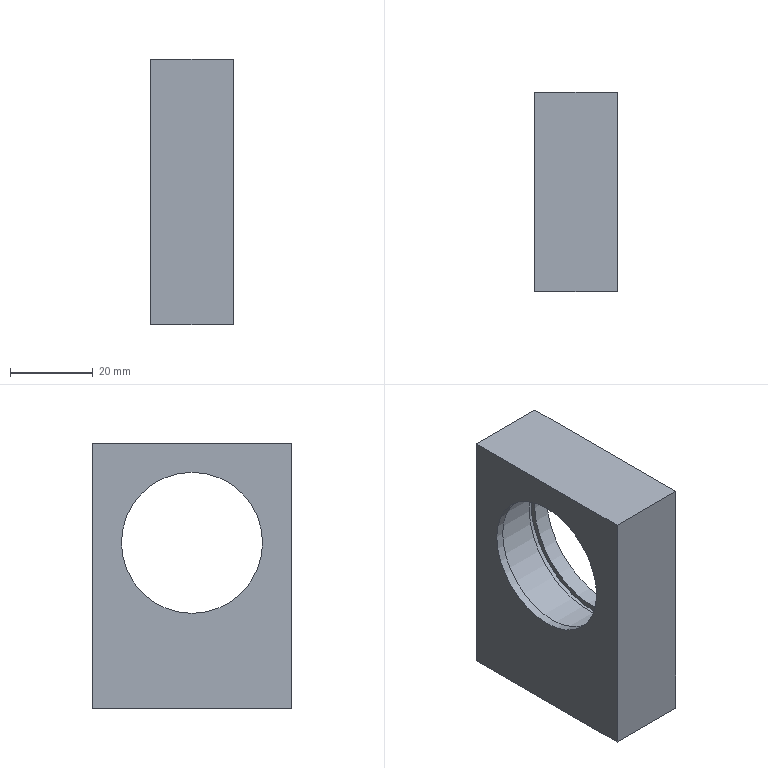Part | NX | features Housing_5003_010_BGBKB6203ZZ-40 2 | 1 solid | 17 faces | box 20 x 48 x 64 mm | volume 36127 mm3 | plane 9 | cylinder 6 | cone 2 | commonest cylinder face diameters 5 x2 40 x2 34 x1 42.5 x1
STEP:
#1=CARTESIAN_POINT('',(171.525,100.,-123.));
#2=VERTEX_POINT('',#1);
#3=CARTESIAN_POINT('',(171.525,100.,-187.));
#4=VERTEX_POINT('',#3);
#5=CARTESIAN_POINT('',(171.525,100.,-187.));
#6=DIRECTION('',(0.,0.,-1.));
#7=VECTOR('',#6,1000.);
#8=LINE('',#5,#7);
#9=EDGE_CURVE('',#2,#4,#8,.T.);
#10=ORIENTED_EDGE('',*,*,#9,.T.);
#11=CARTESIAN_POINT('',(191.525,100.,-187.));
#12=VERTEX_POINT('',#11);
#13=CARTESIAN_POINT('',(191.525,100.,-187.));
#14=DIRECTION('',(-1.,0.,0.));
#15=VECTOR('',#14,1000.);
#16=LINE('',#13,#15);
#17=EDGE_CURVE('',#12,#4,#16,.T.);
#18=ORIENTED_EDGE('',*,*,#17,.F.);
#19=CARTESIAN_POINT('',(191.525,100.,-123.));
#20=VERTEX_POINT('',#19);
#21=CARTESIAN_POINT('',(191.525,100.,-187.));
#22=DIRECTION('',(0.,0.,-1.));
#23=VECTOR('',#22,1000.);
#24=LINE('',#21,#23);
#25=EDGE_CURVE('',#20,#12,#24,.T.);
#26=ORIENTED_EDGE('',*,*,#25,.F.);
#27=CARTESIAN_POINT('',(191.525,100.,-123.));
#28=DIRECTION('',(-1.,0.,0.));
#29=VECTOR('',#28,1000.);
#30=LINE('',#27,#29);
#31=EDGE_CURVE('',#20,#2,#30,.T.);
#32=ORIENTED_EDGE('',*,*,#31,.T.);
#33=EDGE_LOOP('',(#10,#18,#26,#32));
#34=FACE_BOUND('',#33,.T.);
#35=CARTESIAN_POINT('',(191.525,100.,-187.));
#36=DIRECTION('',(0.,1.,0.));
#37=DIRECTION('',(-1.,0.,0.));
#38=AXIS2_PLACEMENT_3D('',#35,#36,#37);
#39=PLANE('',#38);
#40=ADVANCED_FACE('',(#34),#39,.F.);
#41=CARTESIAN_POINT('',(179.025,142.,-187.));
#42=VERTEX_POINT('',#41);
#43=CARTESIAN_POINT('',(181.525,142.,-187.));
#44=DIRECTION('',(0.,0.,-1.));
#45=DIRECTION('',(-1.,0.,0.));
#46=AXIS2_PLACEMENT_3D('',#43,#44,#45);
#47=CIRCLE('',#46,2.5);
#48=EDGE_CURVE('',#42,#42,#47,.T.);
#49=ORIENTED_EDGE('',*,*,#48,.F.);
#50=EDGE_LOOP('',(#49));
#51=FACE_BOUND('',#50,.T.);
#52=CARTESIAN_POINT('',(179.025,106.,-187.));
#53=VERTEX_POINT('',#52);
#54=CARTESIAN_POINT('',(181.525,106.,-187.));
#55=DIRECTION('',(0.,0.,-1.));
#56=DIRECTION('',(-1.,0.,0.));
#57=AXIS2_PLACEMENT_3D('',#54,#55,#56);
#58=CIRCLE('',#57,2.5);
#59=EDGE_CURVE('',#53,#53,#58,.T.);
#60=ORIENTED_EDGE('',*,*,#59,.F.);
#61=EDGE_LOOP('',(#60));
#62=FACE_BOUND('',#61,.T.);
#63=CARTESIAN_POINT('',(171.525,148.,-187.));
#64=VERTEX_POINT('',#63);
#65=CARTESIAN_POINT('',(171.525,100.,-187.));
#66=DIRECTION('',(0.,1.,0.));
#67=VECTOR('',#66,1000.);
#68=LINE('',#65,#67);
#69=EDGE_CURVE('',#4,#64,#68,.T.);
#70=ORIENTED_EDGE('',*,*,#69,.T.);
#71=CARTESIAN_POINT('',(191.525,148.,-187.));
#72=VERTEX_POINT('',#71);
#73=CARTESIAN_POINT('',(191.525,148.,-187.));
#74=DIRECTION('',(-1.,0.,0.));
#75=VECTOR('',#74,1000.);
#76=LINE('',#73,#75);
#77=EDGE_CURVE('',#72,#64,#76,.T.);
#78=ORIENTED_EDGE('',*,*,#77,.F.);
#79=CARTESIAN_POINT('',(191.525,100.,-187.));
#80=DIRECTION('',(0.,1.,0.));
#81=VECTOR('',#80,1000.);
#82=LINE('',#79,#81);
#83=EDGE_CURVE('',#12,#72,#82,.T.);
#84=ORIENTED_EDGE('',*,*,#83,.F.);
#85=ORIENTED_EDGE('',*,*,#17,.T.);
#86=EDGE_LOOP('',(#70,#78,#84,#85));
#87=FACE_BOUND('',#86,.T.);
#88=CARTESIAN_POINT('',(191.525,100.,-187.));
#89=DIRECTION('',(0.,0.,1.));
#90=DIRECTION('',(1.,0.,0.));
#91=AXIS2_PLACEMENT_3D('',#88,#89,#90);
#92=PLANE('',#91);
#93=ADVANCED_FACE('',(#51,#62,#87),#92,.F.);
#94=CARTESIAN_POINT('',(171.525,148.,-123.));
#95=VERTEX_POINT('',#94);
#96=CARTESIAN_POINT('',(171.525,148.,-187.));
#97=DIRECTION('',(0.,0.,1.));
#98=VECTOR('',#97,1000.);
#99=LINE('',#96,#98);
#100=EDGE_CURVE('',#64,#95,#99,.T.);
#101=ORIENTED_EDGE('',*,*,#100,.T.);
#102=CARTESIAN_POINT('',(191.525,148.,-123.));
#103=VERTEX_POINT('',#102);
#104=CARTESIAN_POINT('',(191.525,148.,-123.));
#105=DIRECTION('',(-1.,0.,0.));
#106=VECTOR('',#105,1000.);
#107=LINE('',#104,#106);
#108=EDGE_CURVE('',#103,#95,#107,.T.);
#109=ORIENTED_EDGE('',*,*,#108,.F.);
#110=CARTESIAN_POINT('',(191.525,148.,-187.));
#111=DIRECTION('',(0.,0.,1.));
#112=VECTOR('',#111,1000.);
#113=LINE('',#110,#112);
#114=EDGE_CURVE('',#72,#103,#113,.T.);
#115=ORIENTED_EDGE('',*,*,#114,.F.);
#116=ORIENTED_EDGE('',*,*,#77,.T.);
#117=EDGE_LOOP('',(#101,#109,#115,#116));
#118=FACE_BOUND('',#117,.T.);
#119=CARTESIAN_POINT('',(191.525,148.,-187.));
#120=DIRECTION('',(0.,-1.,0.));
#121=DIRECTION('',(1.,0.,0.));
#122=AXIS2_PLACEMENT_3D('',#119,#120,#121);
#123=PLANE('',#122);
#124=ADVANCED_FACE('',(#118),#123,.F.);
#125=CARTESIAN_POINT('',(171.525,100.,-123.));
#126=DIRECTION('',(0.,-1.,0.));
#127=VECTOR('',#126,1000.);
#128=LINE('',#125,#127);
#129=EDGE_CURVE('',#95,#2,#128,.T.);
#130=ORIENTED_EDGE('',*,*,#129,.T.);
#131=ORIENTED_EDGE('',*,*,#31,.F.);
#132=CARTESIAN_POINT('',(191.525,100.,-123.));
#133=DIRECTION('',(0.,-1.,0.));
#134=VECTOR('',#133,1000.);
#135=LINE('',#132,#134);
#136=EDGE_CURVE('',#103,#20,#135,.T.);
#137=ORIENTED_EDGE('',*,*,#136,.F.);
#138=ORIENTED_EDGE('',*,*,#108,.T.);
#139=EDGE_LOOP('',(#130,#131,#137,#138));
#140=FACE_BOUND('',#139,.T.);
#141=CARTESIAN_POINT('',(191.525,100.,-123.));
#142=DIRECTION('',(0.,0.,-1.));
#143=DIRECTION('',(-1.,0.,0.));
#144=AXIS2_PLACEMENT_3D('',#141,#142,#143);
#145=PLANE('',#144);
#146=ADVANCED_FACE('',(#140),#145,.F.);
#147=CARTESIAN_POINT('',(191.525,124.,-127.));
#148=VERTEX_POINT('',#147);
#149=CARTESIAN_POINT('',(191.525,124.,-147.));
#150=DIRECTION('',(-1.,0.,0.));
#151=DIRECTION('',(0.,0.,1.));
#152=AXIS2_PLACEMENT_3D('',#149,#150,#151);
#153=CIRCLE('',#152,20.);
#154=EDGE_CURVE('',#148,#148,#153,.T.);
#155=ORIENTED_EDGE('',*,*,#154,.T.);
#156=EDGE_LOOP('',(#155));
#157=FACE_BOUND('',#156,.T.);
#158=ORIENTED_EDGE('',*,*,#25,.T.);
#159=ORIENTED_EDGE('',*,*,#83,.T.);
#160=ORIENTED_EDGE('',*,*,#114,.T.);
#161=ORIENTED_EDGE('',*,*,#136,.T.);
#162=EDGE_LOOP('',(#158,#159,#160,#161));
#163=FACE_BOUND('',#162,.T.);
#164=CARTESIAN_POINT('',(191.525,124.,-187.));
#165=DIRECTION('',(-1.,0.,0.));
#166=DIRECTION('',(0.,-1.,0.));
#167=AXIS2_PLACEMENT_3D('',#164,#165,#166);
#168=PLANE('',#167);
#169=ADVANCED_FACE('',(#157,#163),#168,.F.);
#170=CARTESIAN_POINT('',(171.525,124.,-130.));
#171=VERTEX_POINT('',#170);
#172=CARTESIAN_POINT('',(171.525,124.,-147.));
#173=DIRECTION('',(-1.,0.,0.));
#174=DIRECTION('',(0.,0.,1.));
#175=AXIS2_PLACEMENT_3D('',#172,#173,#174);
#176=CIRCLE('',#175,17.);
#177=EDGE_CURVE('',#171,#171,#176,.T.);
#178=ORIENTED_EDGE('',*,*,#177,.F.);
#179=EDGE_LOOP('',(#178));
#180=FACE_BOUND('',#179,.T.);
#181=ORIENTED_EDGE('',*,*,#9,.F.);
#182=ORIENTED_EDGE('',*,*,#129,.F.);
#183=ORIENTED_EDGE('',*,*,#100,.F.);
#184=ORIENTED_EDGE('',*,*,#69,.F.);
#185=EDGE_LOOP('',(#181,#182,#183,#184));
#186=FACE_BOUND('',#185,.T.);
#187=CARTESIAN_POINT('',(171.525,124.,-187.));
#188=DIRECTION('',(-1.,0.,0.));
#189=DIRECTION('',(0.,-1.,0.));
#190=AXIS2_PLACEMENT_3D('',#187,#188,#189);
#191=PLANE('',#190);
#192=ADVANCED_FACE('',(#180,#186),#191,.T.);
#193=CARTESIAN_POINT('',(173.525,124.,-130.));
#194=VERTEX_POINT('',#193);
#195=CARTESIAN_POINT('',(173.525,124.,-147.));
#196=DIRECTION('',(-1.,0.,0.));
#197=DIRECTION('',(0.,0.,1.));
#198=AXIS2_PLACEMENT_3D('',#195,#196,#197);
#199=CIRCLE('',#198,17.);
#200=EDGE_CURVE('',#194,#194,#199,.T.);
#201=ORIENTED_EDGE('',*,*,#200,.F.);
#202=EDGE_LOOP('',(#201));
#203=FACE_BOUND('',#202,.T.);
#204=ORIENTED_EDGE('',*,*,#177,.T.);
#205=EDGE_LOOP('',(#204));
#206=FACE_BOUND('',#205,.T.);
#207=CARTESIAN_POINT('',(171.525,124.,-147.));
#208=DIRECTION('',(-1.,0.,0.));
#209=DIRECTION('',(0.,0.,1.));
#210=AXIS2_PLACEMENT_3D('',#207,#208,#209);
#211=CYLINDRICAL_SURFACE('',#210,17.);
#212=ADVANCED_FACE('',(#203,#206),#211,.F.);
#213=CARTESIAN_POINT('',(173.525,124.,-127.));
#214=VERTEX_POINT('',#213);
#215=CARTESIAN_POINT('',(173.525,124.,-147.));
#216=DIRECTION('',(-1.,0.,0.));
#217=DIRECTION('',(0.,0.,1.));
#218=AXIS2_PLACEMENT_3D('',#215,#216,#217);
#219=CIRCLE('',#218,20.);
#220=EDGE_CURVE('',#214,#214,#219,.T.);
#221=ORIENTED_EDGE('',*,*,#220,.F.);
#222=EDGE_LOOP('',(#221));
#223=FACE_BOUND('',#222,.T.);
#224=ORIENTED_EDGE('',*,*,#200,.T.);
#225=EDGE_LOOP('',(#224));
#226=FACE_BOUND('',#225,.T.);
#227=CARTESIAN_POINT('',(173.525,124.,-130.));
#228=DIRECTION('',(-1.,0.,0.));
#229=DIRECTION('',(0.,0.,1.));
#230=AXIS2_PLACEMENT_3D('',#227,#228,#229);
#231=PLANE('',#230);
#232=ADVANCED_FACE('',(#223,#226),#231,.F.);
#233=CARTESIAN_POINT('',(185.525,124.,-127.));
#234=VERTEX_POINT('',#233);
#235=CARTESIAN_POINT('',(185.525,124.,-147.));
#236=DIRECTION('',(-1.,0.,0.));
#237=DIRECTION('',(0.,0.,1.));
#238=AXIS2_PLACEMENT_3D('',#235,#236,#237);
#239=CIRCLE('',#238,20.);
#240=EDGE_CURVE('',#234,#234,#239,.T.);
#241=ORIENTED_EDGE('',*,*,#240,.F.);
#242=EDGE_LOOP('',(#241));
#243=FACE_BOUND('',#242,.T.);
#244=ORIENTED_EDGE('',*,*,#220,.T.);
#245=EDGE_LOOP('',(#244));
#246=FACE_BOUND('',#245,.T.);
#247=CARTESIAN_POINT('',(171.525,124.,-147.));
#248=DIRECTION('',(-1.,0.,0.));
#249=DIRECTION('',(0.,0.,1.));
#250=AXIS2_PLACEMENT_3D('',#247,#248,#249);
#251=CYLINDRICAL_SURFACE('',#250,20.);
#252=ADVANCED_FACE('',(#243,#246),#251,.F.);
#253=CARTESIAN_POINT('',(185.525,124.,-125.75));
#254=VERTEX_POINT('',#253);
#255=CARTESIAN_POINT('',(185.525,124.,-147.));
#256=DIRECTION('',(-1.,0.,0.));
#257=DIRECTION('',(0.,0.,1.));
#258=AXIS2_PLACEMENT_3D('',#255,#256,#257);
#259=CIRCLE('',#258,21.25);
#260=EDGE_CURVE('',#254,#254,#259,.T.);
#261=ORIENTED_EDGE('',*,*,#260,.F.);
#262=EDGE_LOOP('',(#261));
#263=FACE_BOUND('',#262,.T.);
#264=ORIENTED_EDGE('',*,*,#240,.T.);
#265=EDGE_LOOP('',(#264));
#266=FACE_BOUND('',#265,.T.);
#267=CARTESIAN_POINT('',(185.525,124.,-127.));
#268=DIRECTION('',(-1.,0.,0.));
#269=DIRECTION('',(0.,0.,1.));
#270=AXIS2_PLACEMENT_3D('',#267,#268,#269);
#271=PLANE('',#270);
#272=ADVANCED_FACE('',(#263,#266),#271,.F.);
#273=CARTESIAN_POINT('',(187.425,124.,-125.75));
#274=VERTEX_POINT('',#273);
#275=CARTESIAN_POINT('',(187.425,124.,-147.));
#276=DIRECTION('',(-1.,0.,0.));
#277=DIRECTION('',(0.,0.,1.));
#278=AXIS2_PLACEMENT_3D('',#275,#276,#277);
#279=CIRCLE('',#278,21.25);
#280=EDGE_CURVE('',#274,#274,#279,.T.);
#281=ORIENTED_EDGE('',*,*,#280,.F.);
#282=EDGE_LOOP('',(#281));
#283=FACE_BOUND('',#282,.T.);
#284=ORIENTED_EDGE('',*,*,#260,.T.);
#285=EDGE_LOOP('',(#284));
#286=FACE_BOUND('',#285,.T.);
#287=CARTESIAN_POINT('',(171.525,124.,-147.));
#288=DIRECTION('',(-1.,0.,0.));
#289=DIRECTION('',(0.,0.,1.));
#290=AXIS2_PLACEMENT_3D('',#287,#288,#289);
#291=CYLINDRICAL_SURFACE('',#290,21.25);
#292=ADVANCED_FACE('',(#283,#286),#291,.F.);
#293=CARTESIAN_POINT('',(187.425,124.,-127.));
#294=VERTEX_POINT('',#293);
#295=CARTESIAN_POINT('',(187.425,124.,-147.));
#296=DIRECTION('',(-1.,0.,0.));
#297=DIRECTION('',(0.,0.,1.));
#298=AXIS2_PLACEMENT_3D('',#295,#296,#297);
#299=CIRCLE('',#298,20.);
#300=EDGE_CURVE('',#294,#294,#299,.T.);
#301=ORIENTED_EDGE('',*,*,#300,.F.);
#302=EDGE_LOOP('',(#301));
#303=FACE_BOUND('',#302,.T.);
#304=ORIENTED_EDGE('',*,*,#280,.T.);
#305=EDGE_LOOP('',(#304));
#306=FACE_BOUND('',#305,.T.);
#307=CARTESIAN_POINT('',(187.425,124.,-125.75));
#308=DIRECTION('',(1.,0.,0.));
#309=DIRECTION('',(0.,0.,-1.));
#310=AXIS2_PLACEMENT_3D('',#307,#308,#309);
#311=PLANE('',#310);
#312=ADVANCED_FACE('',(#303,#306),#311,.F.);
#313=ORIENTED_EDGE('',*,*,#154,.F.);
#314=EDGE_LOOP('',(#313));
#315=FACE_BOUND('',#314,.T.);
#316=ORIENTED_EDGE('',*,*,#300,.T.);
#317=EDGE_LOOP('',(#316));
#318=FACE_BOUND('',#317,.T.);
#319=CARTESIAN_POINT('',(171.525,124.,-147.));
#320=DIRECTION('',(-1.,0.,0.));
#321=DIRECTION('',(0.,0.,1.));
#322=AXIS2_PLACEMENT_3D('',#319,#320,#321);
#323=CYLINDRICAL_SURFACE('',#322,20.);
#324=ADVANCED_FACE('',(#315,#318),#323,.F.);
#325=CARTESIAN_POINT('',(181.525,106.,-171.498));
#326=VERTEX_POINT('',#325);
#327=VERTEX_LOOP('',#326);
#328=FACE_BOUND('',#327,.T.);
#329=CARTESIAN_POINT('',(179.025,106.,-173.));
#330=VERTEX_POINT('',#329);
#331=CARTESIAN_POINT('',(181.525,106.,-173.));
#332=DIRECTION('',(0.,0.,-1.));
#333=DIRECTION('',(-1.,0.,0.));
#334=AXIS2_PLACEMENT_3D('',#331,#332,#333);
#335=CIRCLE('',#334,2.5);
#336=EDGE_CURVE('',#330,#330,#335,.T.);
#337=ORIENTED_EDGE('',*,*,#336,.T.);
#338=EDGE_LOOP('',(#337));
#339=FACE_BOUND('',#338,.T.);
#340=CARTESIAN_POINT('',(181.525,106.,-173.));
#341=DIRECTION('',(0.,0.,-1.));
#342=DIRECTION('',(-1.,0.,0.));
#343=AXIS2_PLACEMENT_3D('',#340,#341,#342);
#344=CONICAL_SURFACE('',#343,2.5,1.03);
#345=ADVANCED_FACE('',(#328,#339),#344,.F.);
#346=ORIENTED_EDGE('',*,*,#336,.F.);
#347=EDGE_LOOP('',(#346));
#348=FACE_BOUND('',#347,.T.);
#349=ORIENTED_EDGE('',*,*,#59,.T.);
#350=EDGE_LOOP('',(#349));
#351=FACE_BOUND('',#350,.T.);
#352=CARTESIAN_POINT('',(181.525,106.,-187.));
#353=DIRECTION('',(0.,0.,-1.));
#354=DIRECTION('',(-1.,0.,0.));
#355=AXIS2_PLACEMENT_3D('',#352,#353,#354);
#356=CYLINDRICAL_SURFACE('',#355,2.5);
#357=ADVANCED_FACE('',(#348,#351),#356,.F.);
#358=CARTESIAN_POINT('',(181.525,142.,-171.498));
#359=VERTEX_POINT('',#358);
#360=VERTEX_LOOP('',#359);
#361=FACE_BOUND('',#360,.T.);
#362=CARTESIAN_POINT('',(179.025,142.,-173.));
#363=VERTEX_POINT('',#362);
#364=CARTESIAN_POINT('',(181.525,142.,-173.));
#365=DIRECTION('',(0.,0.,-1.));
#366=DIRECTION('',(-1.,0.,0.));
#367=AXIS2_PLACEMENT_3D('',#364,#365,#366);
#368=CIRCLE('',#367,2.5);
#369=EDGE_CURVE('',#363,#363,#368,.T.);
#370=ORIENTED_EDGE('',*,*,#369,.T.);
#371=EDGE_LOOP('',(#370));
#372=FACE_BOUND('',#371,.T.);
#373=CARTESIAN_POINT('',(181.525,142.,-173.));
#374=DIRECTION('',(0.,0.,-1.));
#375=DIRECTION('',(-1.,0.,0.));
#376=AXIS2_PLACEMENT_3D('',#373,#374,#375);
#377=CONICAL_SURFACE('',#376,2.5,1.03);
#378=ADVANCED_FACE('',(#361,#372),#377,.F.);
#379=ORIENTED_EDGE('',*,*,#369,.F.);
#380=EDGE_LOOP('',(#379));
#381=FACE_BOUND('',#380,.T.);
#382=ORIENTED_EDGE('',*,*,#48,.T.);
#383=EDGE_LOOP('',(#382));
#384=FACE_BOUND('',#383,.T.);
#385=CARTESIAN_POINT('',(181.525,142.,-187.));
#386=DIRECTION('',(0.,0.,-1.));
#387=DIRECTION('',(-1.,0.,0.));
#388=AXIS2_PLACEMENT_3D('',#385,#386,#387);
#389=CYLINDRICAL_SURFACE('',#388,2.5);
#390=ADVANCED_FACE('',(#381,#384),#389,.F.);
#391=CLOSED_SHELL('',(#40,#93,#124,#146,#169,#192,#212,#232,#252,#272,#292,#312,#324,#345,#357,#378,#390));
#392=MANIFOLD_SOLID_BREP('',#391);
#393=(LENGTH_UNIT()NAMED_UNIT(*)SI_UNIT(.MILLI.,.METRE.));
#394=UNCERTAINTY_MEASURE_WITH_UNIT(LENGTH_MEASURE(0.00001),#393,'','');
#395=(NAMED_UNIT(*)PLANE_ANGLE_UNIT()SI_UNIT($,.RADIAN.));
#396=(NAMED_UNIT(*)SI_UNIT($,.STERADIAN.)SOLID_ANGLE_UNIT());
#397=(GEOMETRIC_REPRESENTATION_CONTEXT(3)GLOBAL_UNCERTAINTY_ASSIGNED_CONTEXT((#394))GLOBAL_UNIT_ASSIGNED_CONTEXT((#393,#395,#396))REPRESENTATION_CONTEXT('',''));
#398=ADVANCED_BREP_SHAPE_REPRESENTATION('',(#392),#397);